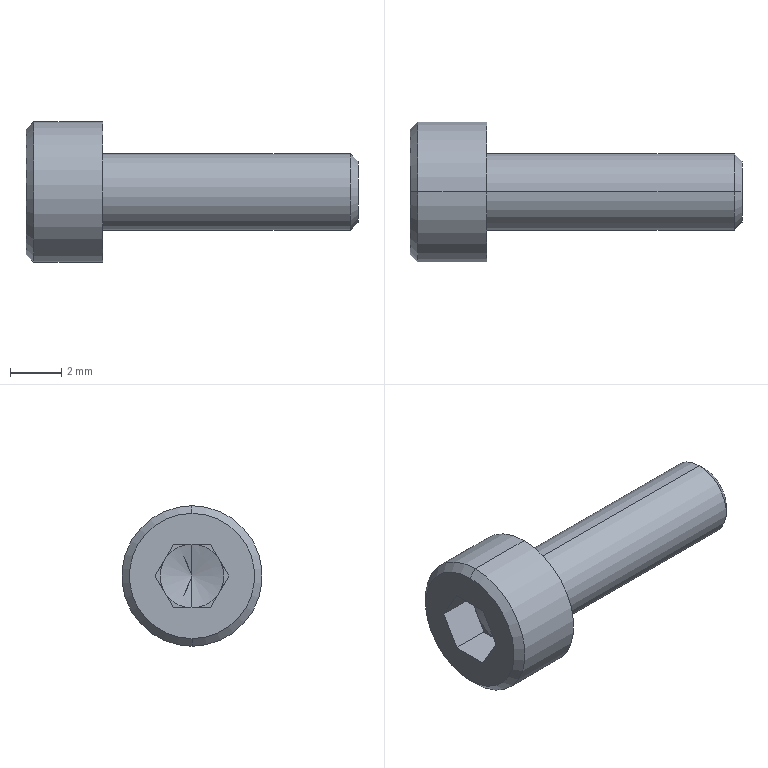Part | STEP file | 0246_302_SCB3-10 | 1 solid | 25 faces | box 13 x 5.5 x 5.5 mm | volume 132.132 mm3 | plane 15 | cone 6 | cylinder 4 | commonest cylinder face diameters 3 x2 5.5 x2